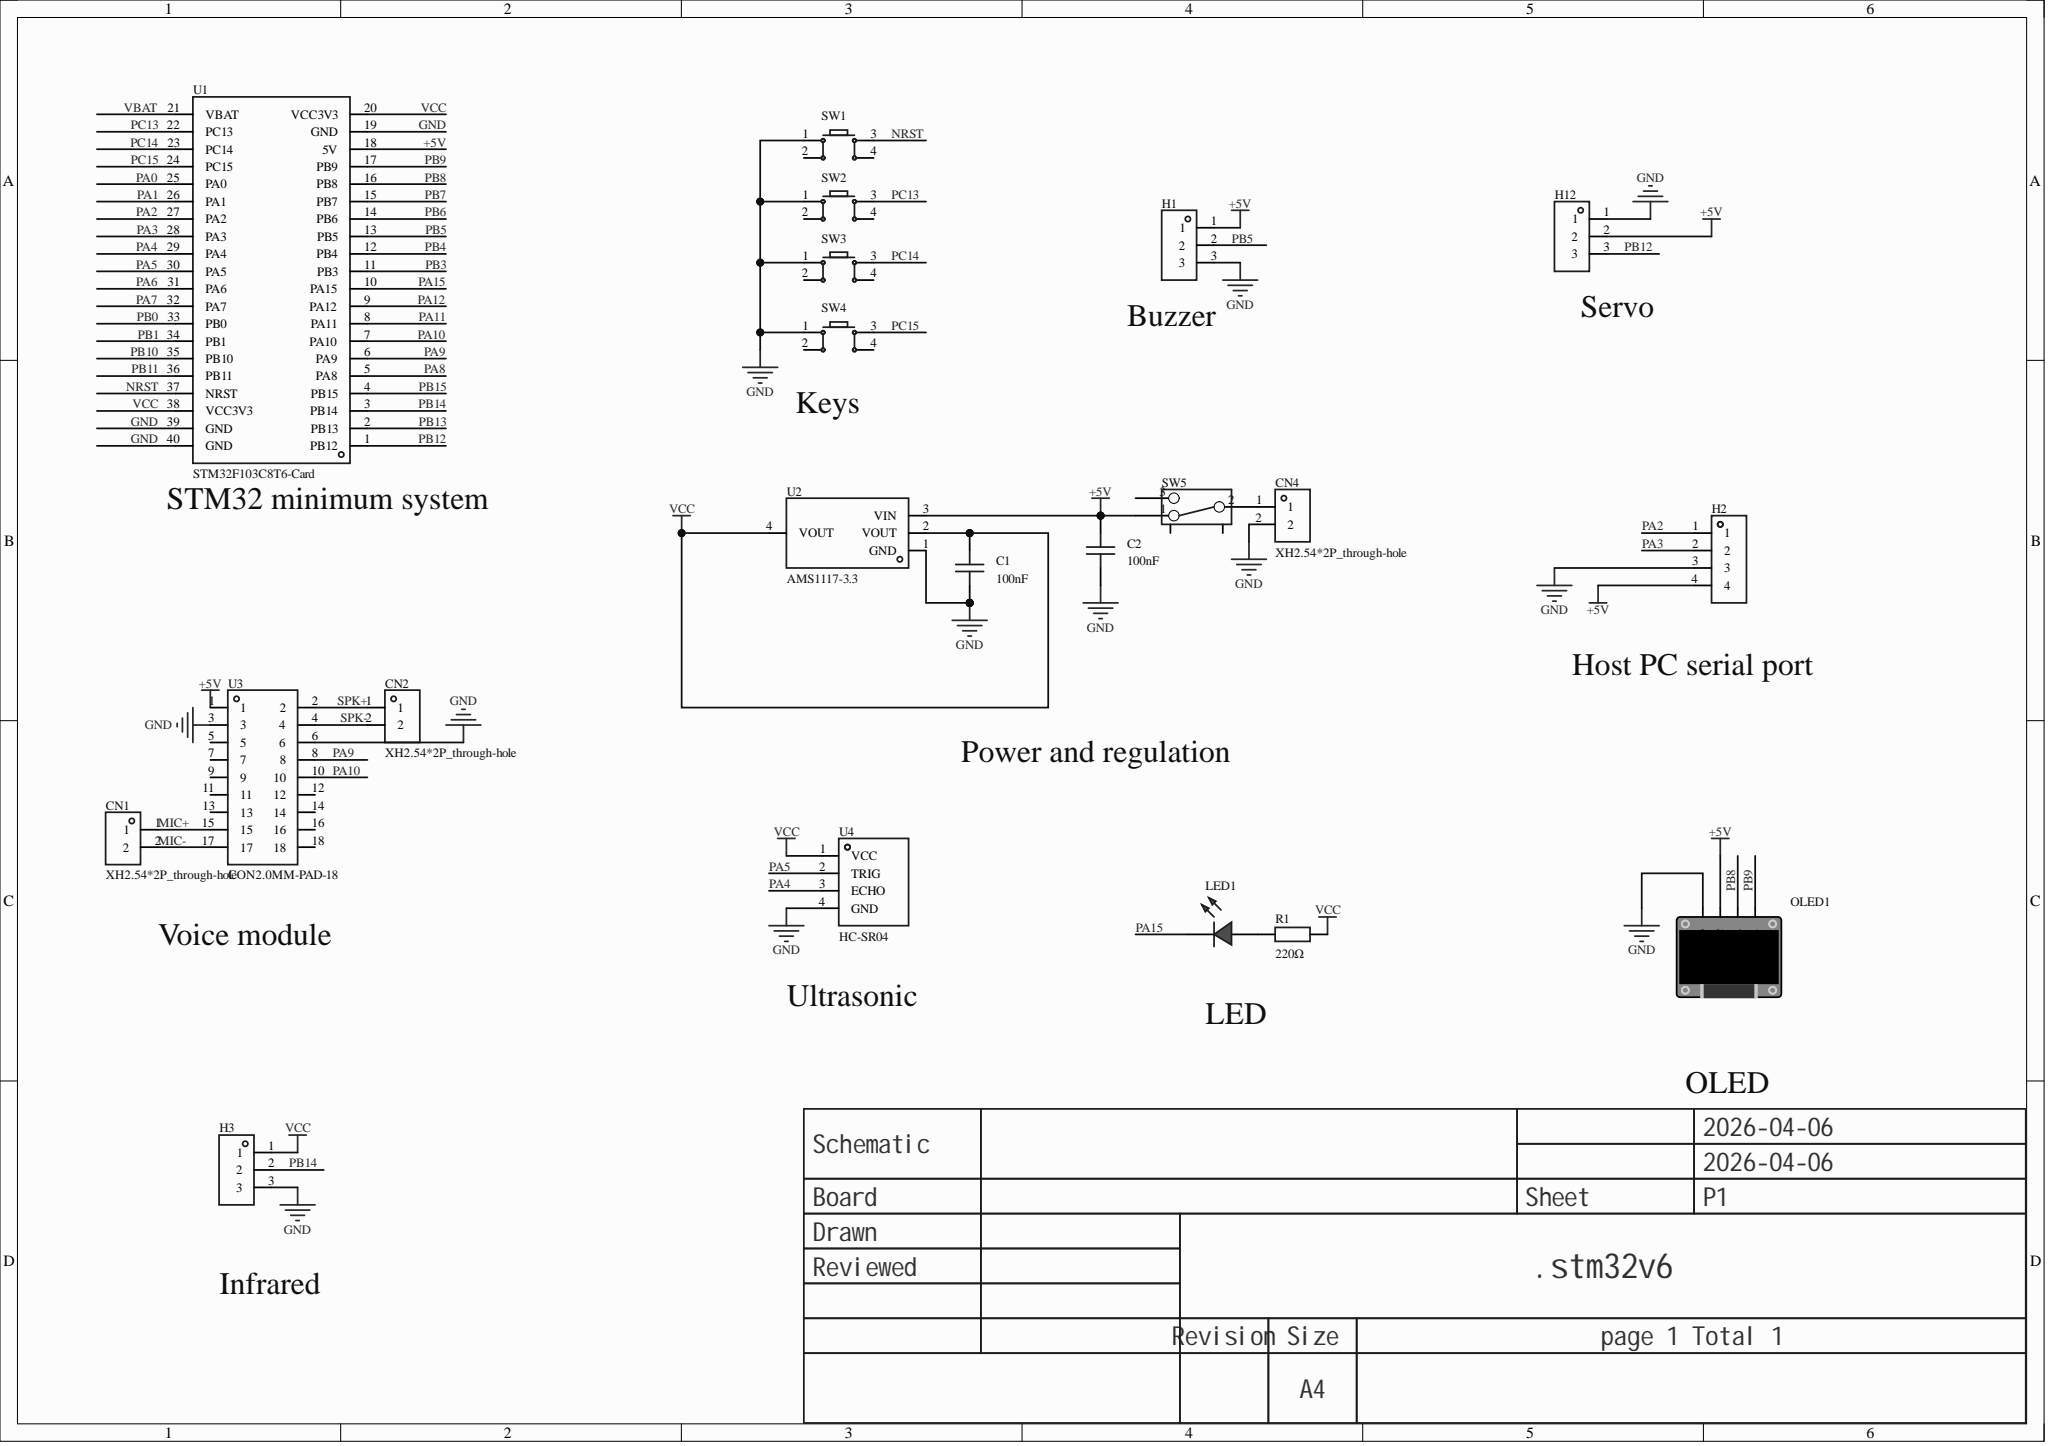Circuit board | Altium Designer | 21 parts | 25 nets
Bill of materials:
Comment,Description,Designator,Footprint,LibRef,Quantity
"100nF","","C1, C2","C0603","CAP_0603","2"
"XH2.54*2P_through-hole","","CN1, CN2, CN4","CONN-TH_2P-P2.50-XH2.54-2P","XH2.54*2P_直插","3"
"","","H1, H3, H12","HDR-TH_3P-P2.54-V-F","HDR-F_2.54_1x3P","3"
"","","H2","HDR-TH_4P-P2.54-V-F","HDR-F_2.54_1x4P","1"
"","","LED1","LED_TH-3mm","LED_TH-R_3mm","1"
"","","OLED1","0.96OLED_4P","0.96OLED模块_4P","1"
"220Ω","","R1","Res_1/8W","Res_AXIAL-1/8W","1"
"","","SW1, SW2, SW3, SW4","SW-TH_4P-L6.0-W6.0-P4.50-LS6.5","Key_TH_6x6x6","4"
"","","SW5","拨动开关","拨动开关_正","1"
"STM32F103C8T6-Card","","U1","CONN-TH_L53.3-W22.9_STM32F103C8T6-CARD","STM32F103C8T6-Card","1"
"AMS1117-3.3","Output type: fixed; working voltage: -; output voltage: 3.3V; output current: 1A; PSRR: 72dB@(120Hz); output polarity: positive;","U2","SOT-223-3_L6.5-W3.4-P2.30-LS7.0-BR","AMS1117-3.3_C6186","1"
"CON2.0MM-PAD-18","","U3","CONN-TH_18P-P2.00_C9900078766","CON2.0MM-PAD-18","1"
"HC-SR04","","U4","TH_HC-SR04V","HC-SR04","1"
Netlist (Protel format):
[
C1
C0603
100nF



]
[
C2
C0603
100nF



]
[
CN1
CONN-TH_2P-P2.50-XH2.54-2P
XH2.54*2P_through-hole



]
[
CN2
CONN-TH_2P-P2.50-XH2.54-2P
XH2.54*2P_through-hole



]
[
CN4
CONN-TH_2P-P2.50-XH2.54-2P
XH2.54*2P_through-hole



]
[
H1
HDR-TH_3P-P2.54-V-F




]
[
H2
HDR-TH_4P-P2.54-V-F




]
[
H3
HDR-TH_3P-P2.54-V-F




]
[
H12
HDR-TH_3P-P2.54-V-F




]
[
LED1
LED_TH-3mm




]
[
OLED1
0.96OLED_4P




]
[
R1
Res_1/8W
220Ω



]
[
SW1
SW-TH_4P-L6.0-W6.0-P4.50-LS6.5




]
[
SW2
SW-TH_4P-L6.0-W6.0-P4.50-LS6.5




]
[
SW3
SW-TH_4P-L6.0-W6.0-P4.50-LS6.5




]
[
SW4
SW-TH_4P-L6.0-W6.0-P4.50-LS6.5




]
[
SW5
拨动开关




]
[
U1
CONN-TH_L53.3-W22.9_STM32F103C8T6-CARD
STM32F103C8T6-Card



]
[
U2
SOT-223-3_L6.5-W3.4-P2.30-LS7.0-BR
AMS1117-3.3



]
[
U3
CONN-TH_18P-P2.00_C9900078766
CON2.0MM-PAD-18



]
[
U4
TH_HC-SR04V
HC-SR04



]
(
VCC
C1-2
H3-1
R1-2
U1-20
U1-38
U2-2
U2-4
U4-1
)
(
SPK-
CN2-2
U3-4
)
(
SPK+
CN2-1
U3-2
)
(
PC15
SW4-3
U1-24
)
(
PC14
SW3-3
U1-23
)
(
PC13
SW2-3
U1-22
)
(
PB14
H3-2
U1-3
)
(
PB12
H12-3
U1-1
)
(
PB9
OLED1-4
U1-17
)
(
PB8
OLED1-3
U1-16
)
(
PB5
H1-2
U1-13
)
(
PA15
LED1-2
U1-10
)
(
PA10
U1-7
U3-10
)
(
PA9
U1-6
U3-8
)
(
PA5
U1-30
U4-2
)
(
PA4
U1-29
U4-3
)
(
PA3
H2-2
U1-28
)
(
PA2
H2-1
U1-27
)
(
NRST
SW1-3
U1-37
)
(
NetLED1_1
LED1-1
R1-1
)
(
NetCN4_1
CN4-1
SW5-2
)
(
MIC-
CN1-2
U3-17
)
(
MIC+
CN1-1
U3-15
)
(
GND
C1-1
C2-1
CN4-2
H1-3
H2-3
H3-3
H12-1
OLED1-1
SW1-1
SW2-1
SW3-1
SW4-1
U1-19
U1-39
U1-40
U2-1
U3-3
U3-6
U4-4
)
(
+5V
C2-2
H1-1
H2-4
H12-2
OLED1-2
SW5-1
U1-18
U2-3
U3-1
)